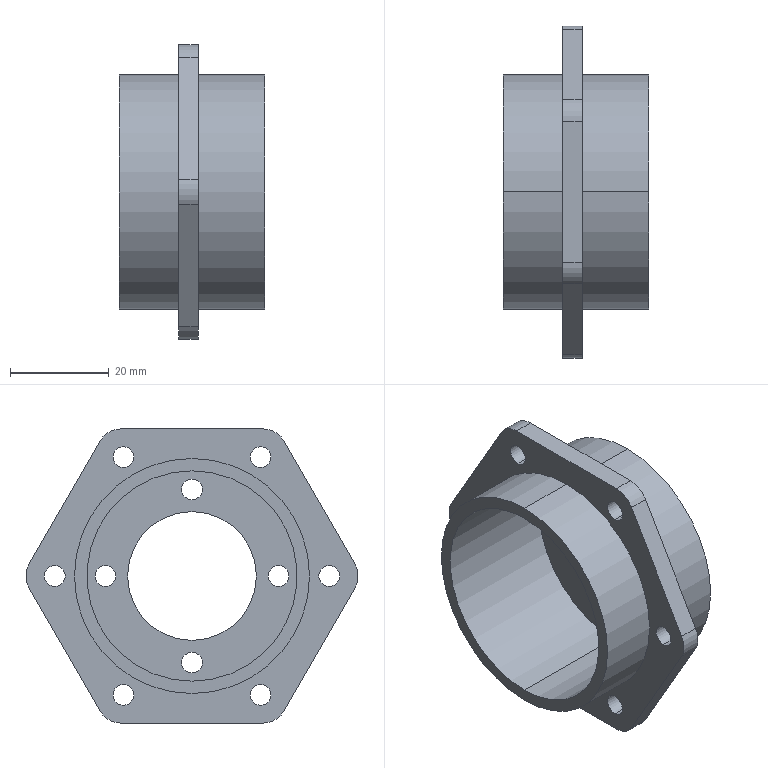Part | SolidWorks | features ICE 3, Fillet 1, Revolution 1 | 1 solid | 45 faces | box 29.45 x 67.158 x 59.5 mm | volume 18545 mm3 | cylinder 34 | plane 11 | commonest cylinder face diameters 4.2 x20 10 x6 47.5 x4 26.02 x2 42.5 x2
STEP:
#1=CARTESIAN_POINT('',(25.45,17.5,2.1));
#2=VERTEX_POINT('',#1);
#3=CARTESIAN_POINT('',(25.45,17.5,-2.1));
#4=VERTEX_POINT('',#3);
#5=CARTESIAN_POINT('',(25.45,17.5,0.));
#6=DIRECTION('',(1.,0.,0.));
#7=DIRECTION('',(0.,0.,-1.));
#8=AXIS2_PLACEMENT_3D('',#5,#6,#7);
#9=CIRCLE('',#8,2.1);
#10=EDGE_CURVE('',#2,#4,#9,.T.);
#11=ORIENTED_EDGE('',*,*,#10,.F.);
#12=CARTESIAN_POINT('',(29.45,17.5,2.1));
#13=VERTEX_POINT('',#12);
#14=CARTESIAN_POINT('',(0.,17.5,2.1));
#15=DIRECTION('',(1.,0.,0.));
#16=VECTOR('',#15,1000.);
#17=LINE('',#14,#16);
#18=EDGE_CURVE('',#2,#13,#17,.T.);
#19=ORIENTED_EDGE('',*,*,#18,.T.);
#20=CARTESIAN_POINT('',(29.45,17.5,-2.1));
#21=VERTEX_POINT('',#20);
#22=CARTESIAN_POINT('',(29.45,17.5,0.));
#23=DIRECTION('',(1.,0.,0.));
#24=DIRECTION('',(0.,0.,-1.));
#25=AXIS2_PLACEMENT_3D('',#22,#23,#24);
#26=CIRCLE('',#25,2.1);
#27=EDGE_CURVE('',#13,#21,#26,.T.);
#28=ORIENTED_EDGE('',*,*,#27,.T.);
#29=CARTESIAN_POINT('',(0.,17.5,-2.1));
#30=DIRECTION('',(1.,0.,0.));
#31=VECTOR('',#30,1000.);
#32=LINE('',#29,#31);
#33=EDGE_CURVE('',#4,#21,#32,.T.);
#34=ORIENTED_EDGE('',*,*,#33,.F.);
#35=EDGE_LOOP('',(#11,#19,#28,#34));
#36=FACE_OUTER_BOUND('',#35,.T.);
#37=CARTESIAN_POINT('',(0.,17.5,0.));
#38=DIRECTION('',(1.,0.,0.));
#39=DIRECTION('',(0.,0.,-1.));
#40=AXIS2_PLACEMENT_3D('',#37,#38,#39);
#41=CYLINDRICAL_SURFACE('',#40,2.1);
#42=ADVANCED_FACE('',(#36),#41,.F.);
#43=CARTESIAN_POINT('',(25.45,0.,-15.4));
#44=VERTEX_POINT('',#43);
#45=CARTESIAN_POINT('',(25.45,0.,-19.6));
#46=VERTEX_POINT('',#45);
#47=CARTESIAN_POINT('',(25.45,0.,-17.5));
#48=DIRECTION('',(1.,0.,0.));
#49=DIRECTION('',(0.,0.,-1.));
#50=AXIS2_PLACEMENT_3D('',#47,#48,#49);
#51=CIRCLE('',#50,2.1);
#52=EDGE_CURVE('',#44,#46,#51,.T.);
#53=ORIENTED_EDGE('',*,*,#52,.F.);
#54=CARTESIAN_POINT('',(29.45,0.,-15.4));
#55=VERTEX_POINT('',#54);
#56=CARTESIAN_POINT('',(0.,0.,-15.4));
#57=DIRECTION('',(1.,0.,0.));
#58=VECTOR('',#57,1000.);
#59=LINE('',#56,#58);
#60=EDGE_CURVE('',#44,#55,#59,.T.);
#61=ORIENTED_EDGE('',*,*,#60,.T.);
#62=CARTESIAN_POINT('',(29.45,0.,-19.6));
#63=VERTEX_POINT('',#62);
#64=CARTESIAN_POINT('',(29.45,0.,-17.5));
#65=DIRECTION('',(1.,0.,0.));
#66=DIRECTION('',(0.,0.,-1.));
#67=AXIS2_PLACEMENT_3D('',#64,#65,#66);
#68=CIRCLE('',#67,2.1);
#69=EDGE_CURVE('',#55,#63,#68,.T.);
#70=ORIENTED_EDGE('',*,*,#69,.T.);
#71=CARTESIAN_POINT('',(0.,0.,-19.6));
#72=DIRECTION('',(1.,0.,0.));
#73=VECTOR('',#72,1000.);
#74=LINE('',#71,#73);
#75=EDGE_CURVE('',#46,#63,#74,.T.);
#76=ORIENTED_EDGE('',*,*,#75,.F.);
#77=EDGE_LOOP('',(#53,#61,#70,#76));
#78=FACE_OUTER_BOUND('',#77,.T.);
#79=CARTESIAN_POINT('',(0.,0.,-17.5));
#80=DIRECTION('',(1.,0.,0.));
#81=DIRECTION('',(0.,0.,-1.));
#82=AXIS2_PLACEMENT_3D('',#79,#80,#81);
#83=CYLINDRICAL_SURFACE('',#82,2.1);
#84=ADVANCED_FACE('',(#78),#83,.F.);
#85=CARTESIAN_POINT('',(25.45,-17.5,2.1));
#86=VERTEX_POINT('',#85);
#87=CARTESIAN_POINT('',(25.45,-17.5,-2.1));
#88=VERTEX_POINT('',#87);
#89=CARTESIAN_POINT('',(25.45,-17.5,0.));
#90=DIRECTION('',(1.,0.,0.));
#91=DIRECTION('',(0.,0.,-1.));
#92=AXIS2_PLACEMENT_3D('',#89,#90,#91);
#93=CIRCLE('',#92,2.1);
#94=EDGE_CURVE('',#86,#88,#93,.T.);
#95=ORIENTED_EDGE('',*,*,#94,.F.);
#96=CARTESIAN_POINT('',(29.45,-17.5,2.1));
#97=VERTEX_POINT('',#96);
#98=CARTESIAN_POINT('',(0.,-17.5,2.1));
#99=DIRECTION('',(1.,0.,0.));
#100=VECTOR('',#99,1000.);
#101=LINE('',#98,#100);
#102=EDGE_CURVE('',#86,#97,#101,.T.);
#103=ORIENTED_EDGE('',*,*,#102,.T.);
#104=CARTESIAN_POINT('',(29.45,-17.5,-2.1));
#105=VERTEX_POINT('',#104);
#106=CARTESIAN_POINT('',(29.45,-17.5,0.));
#107=DIRECTION('',(1.,0.,0.));
#108=DIRECTION('',(0.,0.,-1.));
#109=AXIS2_PLACEMENT_3D('',#106,#107,#108);
#110=CIRCLE('',#109,2.1);
#111=EDGE_CURVE('',#97,#105,#110,.T.);
#112=ORIENTED_EDGE('',*,*,#111,.T.);
#113=CARTESIAN_POINT('',(0.,-17.5,-2.1));
#114=DIRECTION('',(1.,0.,0.));
#115=VECTOR('',#114,1000.);
#116=LINE('',#113,#115);
#117=EDGE_CURVE('',#88,#105,#116,.T.);
#118=ORIENTED_EDGE('',*,*,#117,.F.);
#119=EDGE_LOOP('',(#95,#103,#112,#118));
#120=FACE_OUTER_BOUND('',#119,.T.);
#121=CARTESIAN_POINT('',(0.,-17.5,0.));
#122=DIRECTION('',(1.,0.,0.));
#123=DIRECTION('',(0.,0.,-1.));
#124=AXIS2_PLACEMENT_3D('',#121,#122,#123);
#125=CYLINDRICAL_SURFACE('',#124,2.1);
#126=ADVANCED_FACE('',(#120),#125,.F.);
#127=CARTESIAN_POINT('',(25.45,0.,19.6));
#128=VERTEX_POINT('',#127);
#129=CARTESIAN_POINT('',(25.45,0.,15.4));
#130=VERTEX_POINT('',#129);
#131=CARTESIAN_POINT('',(25.45,0.,17.5));
#132=DIRECTION('',(1.,0.,0.));
#133=DIRECTION('',(0.,0.,-1.));
#134=AXIS2_PLACEMENT_3D('',#131,#132,#133);
#135=CIRCLE('',#134,2.1);
#136=EDGE_CURVE('',#128,#130,#135,.T.);
#137=ORIENTED_EDGE('',*,*,#136,.F.);
#138=CARTESIAN_POINT('',(29.45,0.,19.6));
#139=VERTEX_POINT('',#138);
#140=CARTESIAN_POINT('',(0.,0.,19.6));
#141=DIRECTION('',(1.,0.,0.));
#142=VECTOR('',#141,1000.);
#143=LINE('',#140,#142);
#144=EDGE_CURVE('',#128,#139,#143,.T.);
#145=ORIENTED_EDGE('',*,*,#144,.T.);
#146=CARTESIAN_POINT('',(29.45,0.,15.4));
#147=VERTEX_POINT('',#146);
#148=CARTESIAN_POINT('',(29.45,0.,17.5));
#149=DIRECTION('',(1.,0.,0.));
#150=DIRECTION('',(0.,0.,-1.));
#151=AXIS2_PLACEMENT_3D('',#148,#149,#150);
#152=CIRCLE('',#151,2.1);
#153=EDGE_CURVE('',#139,#147,#152,.T.);
#154=ORIENTED_EDGE('',*,*,#153,.T.);
#155=CARTESIAN_POINT('',(0.,0.,15.4));
#156=DIRECTION('',(1.,0.,0.));
#157=VECTOR('',#156,1000.);
#158=LINE('',#155,#157);
#159=EDGE_CURVE('',#130,#147,#158,.T.);
#160=ORIENTED_EDGE('',*,*,#159,.F.);
#161=EDGE_LOOP('',(#137,#145,#154,#160));
#162=FACE_OUTER_BOUND('',#161,.T.);
#163=CARTESIAN_POINT('',(0.,0.,17.5));
#164=DIRECTION('',(1.,0.,0.));
#165=DIRECTION('',(0.,0.,-1.));
#166=AXIS2_PLACEMENT_3D('',#163,#164,#165);
#167=CYLINDRICAL_SURFACE('',#166,2.1);
#168=ADVANCED_FACE('',(#162),#167,.F.);
#169=CARTESIAN_POINT('',(12.,13.875,-21.932));
#170=VERTEX_POINT('',#169);
#171=CARTESIAN_POINT('',(12.,13.875,-26.132));
#172=VERTEX_POINT('',#171);
#173=CARTESIAN_POINT('',(12.,13.875,-24.032));
#174=DIRECTION('',(1.,0.,0.));
#175=DIRECTION('',(0.,0.,-1.));
#176=AXIS2_PLACEMENT_3D('',#173,#174,#175);
#177=CIRCLE('',#176,2.1);
#178=EDGE_CURVE('',#170,#172,#177,.T.);
#179=ORIENTED_EDGE('',*,*,#178,.F.);
#180=CARTESIAN_POINT('',(16.,13.875,-21.932));
#181=VERTEX_POINT('',#180);
#182=CARTESIAN_POINT('',(0.,13.875,-21.932));
#183=DIRECTION('',(1.,0.,0.));
#184=VECTOR('',#183,1000.);
#185=LINE('',#182,#184);
#186=EDGE_CURVE('',#170,#181,#185,.T.);
#187=ORIENTED_EDGE('',*,*,#186,.T.);
#188=CARTESIAN_POINT('',(16.,13.875,-26.132));
#189=VERTEX_POINT('',#188);
#190=CARTESIAN_POINT('',(16.,13.875,-24.032));
#191=DIRECTION('',(1.,0.,0.));
#192=DIRECTION('',(0.,0.,-1.));
#193=AXIS2_PLACEMENT_3D('',#190,#191,#192);
#194=CIRCLE('',#193,2.1);
#195=EDGE_CURVE('',#181,#189,#194,.T.);
#196=ORIENTED_EDGE('',*,*,#195,.T.);
#197=CARTESIAN_POINT('',(0.,13.875,-26.132));
#198=DIRECTION('',(1.,0.,0.));
#199=VECTOR('',#198,1000.);
#200=LINE('',#197,#199);
#201=EDGE_CURVE('',#172,#189,#200,.T.);
#202=ORIENTED_EDGE('',*,*,#201,.F.);
#203=EDGE_LOOP('',(#179,#187,#196,#202));
#204=FACE_OUTER_BOUND('',#203,.T.);
#205=CARTESIAN_POINT('',(0.,13.875,-24.032));
#206=DIRECTION('',(1.,0.,0.));
#207=DIRECTION('',(0.,0.,-1.));
#208=AXIS2_PLACEMENT_3D('',#205,#206,#207);
#209=CYLINDRICAL_SURFACE('',#208,2.1);
#210=ADVANCED_FACE('',(#204),#209,.F.);
#211=CARTESIAN_POINT('',(12.,-13.875,-21.932));
#212=VERTEX_POINT('',#211);
#213=CARTESIAN_POINT('',(12.,-13.875,-26.132));
#214=VERTEX_POINT('',#213);
#215=CARTESIAN_POINT('',(12.,-13.875,-24.032));
#216=DIRECTION('',(1.,0.,0.));
#217=DIRECTION('',(0.,0.,-1.));
#218=AXIS2_PLACEMENT_3D('',#215,#216,#217);
#219=CIRCLE('',#218,2.1);
#220=EDGE_CURVE('',#212,#214,#219,.T.);
#221=ORIENTED_EDGE('',*,*,#220,.F.);
#222=CARTESIAN_POINT('',(16.,-13.875,-21.932));
#223=VERTEX_POINT('',#222);
#224=CARTESIAN_POINT('',(0.,-13.875,-21.932));
#225=DIRECTION('',(1.,0.,0.));
#226=VECTOR('',#225,1000.);
#227=LINE('',#224,#226);
#228=EDGE_CURVE('',#212,#223,#227,.T.);
#229=ORIENTED_EDGE('',*,*,#228,.T.);
#230=CARTESIAN_POINT('',(16.,-13.875,-26.132));
#231=VERTEX_POINT('',#230);
#232=CARTESIAN_POINT('',(16.,-13.875,-24.032));
#233=DIRECTION('',(1.,0.,0.));
#234=DIRECTION('',(0.,0.,-1.));
#235=AXIS2_PLACEMENT_3D('',#232,#233,#234);
#236=CIRCLE('',#235,2.1);
#237=EDGE_CURVE('',#223,#231,#236,.T.);
#238=ORIENTED_EDGE('',*,*,#237,.T.);
#239=CARTESIAN_POINT('',(0.,-13.875,-26.132));
#240=DIRECTION('',(1.,0.,0.));
#241=VECTOR('',#240,1000.);
#242=LINE('',#239,#241);
#243=EDGE_CURVE('',#214,#231,#242,.T.);
#244=ORIENTED_EDGE('',*,*,#243,.F.);
#245=EDGE_LOOP('',(#221,#229,#238,#244));
#246=FACE_OUTER_BOUND('',#245,.T.);
#247=CARTESIAN_POINT('',(0.,-13.875,-24.032));
#248=DIRECTION('',(1.,0.,0.));
#249=DIRECTION('',(0.,0.,-1.));
#250=AXIS2_PLACEMENT_3D('',#247,#248,#249);
#251=CYLINDRICAL_SURFACE('',#250,2.1);
#252=ADVANCED_FACE('',(#246),#251,.F.);
#253=CARTESIAN_POINT('',(12.,-27.75,2.1));
#254=VERTEX_POINT('',#253);
#255=CARTESIAN_POINT('',(12.,-27.75,-2.1));
#256=VERTEX_POINT('',#255);
#257=CARTESIAN_POINT('',(12.,-27.75,0.));
#258=DIRECTION('',(1.,0.,0.));
#259=DIRECTION('',(0.,0.,-1.));
#260=AXIS2_PLACEMENT_3D('',#257,#258,#259);
#261=CIRCLE('',#260,2.1);
#262=EDGE_CURVE('',#254,#256,#261,.T.);
#263=ORIENTED_EDGE('',*,*,#262,.F.);
#264=CARTESIAN_POINT('',(16.,-27.75,2.1));
#265=VERTEX_POINT('',#264);
#266=CARTESIAN_POINT('',(0.,-27.75,2.1));
#267=DIRECTION('',(1.,0.,0.));
#268=VECTOR('',#267,1000.);
#269=LINE('',#266,#268);
#270=EDGE_CURVE('',#254,#265,#269,.T.);
#271=ORIENTED_EDGE('',*,*,#270,.T.);
#272=CARTESIAN_POINT('',(16.,-27.75,-2.1));
#273=VERTEX_POINT('',#272);
#274=CARTESIAN_POINT('',(16.,-27.75,0.));
#275=DIRECTION('',(1.,0.,0.));
#276=DIRECTION('',(0.,0.,-1.));
#277=AXIS2_PLACEMENT_3D('',#274,#275,#276);
#278=CIRCLE('',#277,2.1);
#279=EDGE_CURVE('',#265,#273,#278,.T.);
#280=ORIENTED_EDGE('',*,*,#279,.T.);
#281=CARTESIAN_POINT('',(0.,-27.75,-2.1));
#282=DIRECTION('',(1.,0.,0.));
#283=VECTOR('',#282,1000.);
#284=LINE('',#281,#283);
#285=EDGE_CURVE('',#256,#273,#284,.T.);
#286=ORIENTED_EDGE('',*,*,#285,.F.);
#287=EDGE_LOOP('',(#263,#271,#280,#286));
#288=FACE_OUTER_BOUND('',#287,.T.);
#289=CARTESIAN_POINT('',(0.,-27.75,0.));
#290=DIRECTION('',(1.,0.,0.));
#291=DIRECTION('',(0.,0.,-1.));
#292=AXIS2_PLACEMENT_3D('',#289,#290,#291);
#293=CYLINDRICAL_SURFACE('',#292,2.1);
#294=ADVANCED_FACE('',(#288),#293,.F.);
#295=CARTESIAN_POINT('',(12.,-13.875,26.132));
#296=VERTEX_POINT('',#295);
#297=CARTESIAN_POINT('',(12.,-13.875,21.932));
#298=VERTEX_POINT('',#297);
#299=CARTESIAN_POINT('',(12.,-13.875,24.032));
#300=DIRECTION('',(1.,0.,0.));
#301=DIRECTION('',(0.,0.,-1.));
#302=AXIS2_PLACEMENT_3D('',#299,#300,#301);
#303=CIRCLE('',#302,2.1);
#304=EDGE_CURVE('',#296,#298,#303,.T.);
#305=ORIENTED_EDGE('',*,*,#304,.F.);
#306=CARTESIAN_POINT('',(16.,-13.875,26.132));
#307=VERTEX_POINT('',#306);
#308=CARTESIAN_POINT('',(0.,-13.875,26.132));
#309=DIRECTION('',(1.,0.,0.));
#310=VECTOR('',#309,1000.);
#311=LINE('',#308,#310);
#312=EDGE_CURVE('',#296,#307,#311,.T.);
#313=ORIENTED_EDGE('',*,*,#312,.T.);
#314=CARTESIAN_POINT('',(16.,-13.875,21.932));
#315=VERTEX_POINT('',#314);
#316=CARTESIAN_POINT('',(16.,-13.875,24.032));
#317=DIRECTION('',(1.,0.,0.));
#318=DIRECTION('',(0.,0.,-1.));
#319=AXIS2_PLACEMENT_3D('',#316,#317,#318);
#320=CIRCLE('',#319,2.1);
#321=EDGE_CURVE('',#307,#315,#320,.T.);
#322=ORIENTED_EDGE('',*,*,#321,.T.);
#323=CARTESIAN_POINT('',(0.,-13.875,21.932));
#324=DIRECTION('',(1.,0.,0.));
#325=VECTOR('',#324,1000.);
#326=LINE('',#323,#325);
#327=EDGE_CURVE('',#298,#315,#326,.T.);
#328=ORIENTED_EDGE('',*,*,#327,.F.);
#329=EDGE_LOOP('',(#305,#313,#322,#328));
#330=FACE_OUTER_BOUND('',#329,.T.);
#331=CARTESIAN_POINT('',(0.,-13.875,24.032));
#332=DIRECTION('',(1.,0.,0.));
#333=DIRECTION('',(0.,0.,-1.));
#334=AXIS2_PLACEMENT_3D('',#331,#332,#333);
#335=CYLINDRICAL_SURFACE('',#334,2.1);
#336=ADVANCED_FACE('',(#330),#335,.F.);
#337=CARTESIAN_POINT('',(12.,13.875,26.132));
#338=VERTEX_POINT('',#337);
#339=CARTESIAN_POINT('',(12.,13.875,21.932));
#340=VERTEX_POINT('',#339);
#341=CARTESIAN_POINT('',(12.,13.875,24.032));
#342=DIRECTION('',(1.,0.,0.));
#343=DIRECTION('',(0.,0.,-1.));
#344=AXIS2_PLACEMENT_3D('',#341,#342,#343);
#345=CIRCLE('',#344,2.1);
#346=EDGE_CURVE('',#338,#340,#345,.T.);
#347=ORIENTED_EDGE('',*,*,#346,.F.);
#348=CARTESIAN_POINT('',(16.,13.875,26.132));
#349=VERTEX_POINT('',#348);
#350=CARTESIAN_POINT('',(0.,13.875,26.132));
#351=DIRECTION('',(1.,0.,0.));
#352=VECTOR('',#351,1000.);
#353=LINE('',#350,#352);
#354=EDGE_CURVE('',#338,#349,#353,.T.);
#355=ORIENTED_EDGE('',*,*,#354,.T.);
#356=CARTESIAN_POINT('',(16.,13.875,21.932));
#357=VERTEX_POINT('',#356);
#358=CARTESIAN_POINT('',(16.,13.875,24.032));
#359=DIRECTION('',(1.,0.,0.));
#360=DIRECTION('',(0.,0.,-1.));
#361=AXIS2_PLACEMENT_3D('',#358,#359,#360);
#362=CIRCLE('',#361,2.1);
#363=EDGE_CURVE('',#349,#357,#362,.T.);
#364=ORIENTED_EDGE('',*,*,#363,.T.);
#365=CARTESIAN_POINT('',(0.,13.875,21.932));
#366=DIRECTION('',(1.,0.,0.));
#367=VECTOR('',#366,1000.);
#368=LINE('',#365,#367);
#369=EDGE_CURVE('',#340,#357,#368,.T.);
#370=ORIENTED_EDGE('',*,*,#369,.F.);
#371=EDGE_LOOP('',(#347,#355,#364,#370));
#372=FACE_OUTER_BOUND('',#371,.T.);
#373=CARTESIAN_POINT('',(0.,13.875,24.032));
#374=DIRECTION('',(1.,0.,0.));
#375=DIRECTION('',(0.,0.,-1.));
#376=AXIS2_PLACEMENT_3D('',#373,#374,#375);
#377=CYLINDRICAL_SURFACE('',#376,2.1);
#378=ADVANCED_FACE('',(#372),#377,.F.);
#379=CARTESIAN_POINT('',(12.,27.75,2.1));
#380=VERTEX_POINT('',#379);
#381=CARTESIAN_POINT('',(12.,27.75,-2.1));
#382=VERTEX_POINT('',#381);
#383=CARTESIAN_POINT('',(12.,27.75,0.));
#384=DIRECTION('',(1.,0.,0.));
#385=DIRECTION('',(0.,0.,-1.));
#386=AXIS2_PLACEMENT_3D('',#383,#384,#385);
#387=CIRCLE('',#386,2.1);
#388=EDGE_CURVE('',#380,#382,#387,.T.);
#389=ORIENTED_EDGE('',*,*,#388,.F.);
#390=CARTESIAN_POINT('',(16.,27.75,2.1));
#391=VERTEX_POINT('',#390);
#392=CARTESIAN_POINT('',(0.,27.75,2.1));
#393=DIRECTION('',(1.,0.,0.));
#394=VECTOR('',#393,1000.);
#395=LINE('',#392,#394);
#396=EDGE_CURVE('',#380,#391,#395,.T.);
#397=ORIENTED_EDGE('',*,*,#396,.T.);
#398=CARTESIAN_POINT('',(16.,27.75,-2.1));
#399=VERTEX_POINT('',#398);
#400=CARTESIAN_POINT('',(16.,27.75,0.));
#401=DIRECTION('',(1.,0.,0.));
#402=DIRECTION('',(0.,0.,-1.));
#403=AXIS2_PLACEMENT_3D('',#400,#401,#402);
#404=CIRCLE('',#403,2.1);
#405=EDGE_CURVE('',#391,#399,#404,.T.);
#406=ORIENTED_EDGE('',*,*,#405,.T.);
#407=CARTESIAN_POINT('',(0.,27.75,-2.1));
#408=DIRECTION('',(1.,0.,0.));
#409=VECTOR('',#408,1000.);
#410=LINE('',#407,#409);
#411=EDGE_CURVE('',#382,#399,#410,.T.);
#412=ORIENTED_EDGE('',*,*,#411,.F.);
#413=EDGE_LOOP('',(#389,#397,#406,#412));
#414=FACE_OUTER_BOUND('',#413,.T.);
#415=CARTESIAN_POINT('',(0.,27.75,0.));
#416=DIRECTION('',(1.,0.,0.));
#417=DIRECTION('',(0.,0.,-1.));
#418=AXIS2_PLACEMENT_3D('',#415,#416,#417);
#419=CYLINDRICAL_SURFACE('',#418,2.1);
#420=ADVANCED_FACE('',(#414),#419,.F.);
#421=CARTESIAN_POINT('',(29.45,0.,-13.01));
#422=VERTEX_POINT('',#421);
#423=CARTESIAN_POINT('',(29.45,0.,13.01));
#424=VERTEX_POINT('',#423);
#425=CARTESIAN_POINT('',(29.45,0.,0.));
#426=DIRECTION('',(-1.,0.,0.));
#427=DIRECTION('',(0.,0.,1.));
#428=AXIS2_PLACEMENT_3D('',#425,#426,#427);
#429=CIRCLE('',#428,13.01);
#430=EDGE_CURVE('',#422,#424,#429,.T.);
#431=ORIENTED_EDGE('',*,*,#430,.F.);
#432=CARTESIAN_POINT('',(25.45,0.,-13.01));
#433=VERTEX_POINT('',#432);
#434=CARTESIAN_POINT('',(-873.27,0.,-13.01));
#435=DIRECTION('',(-1.,0.,0.));
#436=VECTOR('',#435,1000.);
#437=LINE('',#434,#436);
#438=EDGE_CURVE('',#422,#433,#437,.T.);
#439=ORIENTED_EDGE('',*,*,#438,.T.);
#440=CARTESIAN_POINT('',(25.45,0.,13.01));
#441=VERTEX_POINT('',#440);
#442=CARTESIAN_POINT('',(25.45,0.,0.));
#443=DIRECTION('',(-1.,0.,0.));
#444=DIRECTION('',(0.,0.,1.));
#445=AXIS2_PLACEMENT_3D('',#442,#443,#444);
#446=CIRCLE('',#445,13.01);
#447=EDGE_CURVE('',#433,#441,#446,.T.);
#448=ORIENTED_EDGE('',*,*,#447,.T.);
#449=CARTESIAN_POINT('',(-873.27,0.,13.01));
#450=DIRECTION('',(-1.,0.,0.));
#451=VECTOR('',#450,1000.);
#452=LINE('',#449,#451);
#453=EDGE_CURVE('',#424,#441,#452,.T.);
#454=ORIENTED_EDGE('',*,*,#453,.F.);
#455=EDGE_LOOP('',(#431,#439,#448,#454));
#456=FACE_OUTER_BOUND('',#455,.T.);
#457=CARTESIAN_POINT('',(-873.27,0.,0.));
#458=DIRECTION('',(-1.,0.,0.));
#459=DIRECTION('',(0.,0.,1.));
#460=AXIS2_PLACEMENT_3D('',#457,#458,#459);
#461=CYLINDRICAL_SURFACE('',#460,13.01);
#462=ADVANCED_FACE('',(#456),#461,.F.);
#463=CARTESIAN_POINT('',(29.45,0.,23.75));
#464=VERTEX_POINT('',#463);
#465=CARTESIAN_POINT('',(29.45,0.,-23.75));
#466=VERTEX_POINT('',#465);
#467=CARTESIAN_POINT('',(29.45,0.,0.));
#468=DIRECTION('',(-1.,0.,0.));
#469=DIRECTION('',(0.,0.,1.));
#470=AXIS2_PLACEMENT_3D('',#467,#468,#469);
#471=CIRCLE('',#470,23.75);
#472=EDGE_CURVE('',#464,#466,#471,.T.);
#473=ORIENTED_EDGE('',*,*,#472,.T.);
#474=CARTESIAN_POINT('',(16.,0.,-23.75));
#475=VERTEX_POINT('',#474);
#476=CARTESIAN_POINT('',(-873.27,0.,-23.75));
#477=DIRECTION('',(-1.,0.,0.));
#478=VECTOR('',#477,1000.);
#479=LINE('',#476,#478);
#480=EDGE_CURVE('',#466,#475,#479,.T.);
#481=ORIENTED_EDGE('',*,*,#480,.T.);
#482=CARTESIAN_POINT('',(16.,0.,23.75));
#483=VERTEX_POINT('',#482);
#484=CARTESIAN_POINT('',(16.,0.,0.));
#485=DIRECTION('',(-1.,0.,0.));
#486=DIRECTION('',(0.,0.,1.));
#487=AXIS2_PLACEMENT_3D('',#484,#485,#486);
#488=CIRCLE('',#487,23.75);
#489=EDGE_CURVE('',#483,#475,#488,.T.);
#490=ORIENTED_EDGE('',*,*,#489,.F.);
#491=CARTESIAN_POINT('',(-873.27,0.,23.75));
#492=DIRECTION('',(-1.,0.,0.));
#493=VECTOR('',#492,1000.);
#494=LINE('',#491,#493);
#495=EDGE_CURVE('',#464,#483,#494,.T.);
#496=ORIENTED_EDGE('',*,*,#495,.F.);
#497=EDGE_LOOP('',(#473,#481,#490,#496));
#498=FACE_OUTER_BOUND('',#497,.T.);
#499=CARTESIAN_POINT('',(-873.27,0.,0.));
#500=DIRECTION('',(-1.,0.,0.));
#501=DIRECTION('',(0.,0.,1.));
#502=AXIS2_PLACEMENT_3D('',#499,#500,#501);
#503=CYLINDRICAL_SURFACE('',#502,23.75);
#504=ADVANCED_FACE('',(#498),#503,.T.);
#505=CARTESIAN_POINT('',(12.,0.,23.75));
#506=VERTEX_POINT('',#505);
#507=CARTESIAN_POINT('',(12.,0.,-23.75));
#508=VERTEX_POINT('',#507);
#509=CARTESIAN_POINT('',(12.,0.,0.));
#510=DIRECTION('',(-1.,0.,0.));
#511=DIRECTION('',(0.,0.,1.));
#512=AXIS2_PLACEMENT_3D('',#509,#510,#511);
#513=CIRCLE('',#512,23.75);
#514=EDGE_CURVE('',#506,#508,#513,.T.);
#515=ORIENTED_EDGE('',*,*,#514,.T.);
#516=CARTESIAN_POINT('',(0.,0.,-23.75));
#517=VERTEX_POINT('',#516);
#518=CARTESIAN_POINT('',(-873.27,0.,-23.75));
#519=DIRECTION('',(-1.,0.,0.));
#520=VECTOR('',#519,1000.);
#521=LINE('',#518,#520);
#522=EDGE_CURVE('',#508,#517,#521,.T.);
#523=ORIENTED_EDGE('',*,*,#522,.T.);
#524=CARTESIAN_POINT('',(0.,0.,23.75));
#525=VERTEX_POINT('',#524);
#526=CARTESIAN_POINT('',(0.,0.,0.));
#527=DIRECTION('',(-1.,0.,0.));
#528=DIRECTION('',(0.,0.,1.));
#529=AXIS2_PLACEMENT_3D('',#526,#527,#528);
#530=CIRCLE('',#529,23.75);
#531=EDGE_CURVE('',#525,#517,#530,.T.);
#532=ORIENTED_EDGE('',*,*,#531,.F.);
#533=CARTESIAN_POINT('',(-873.27,0.,23.75));
#534=DIRECTION('',(-1.,0.,0.));
#535=VECTOR('',#534,1000.);
#536=LINE('',#533,#535);
#537=EDGE_CURVE('',#506,#525,#536,.T.);
#538=ORIENTED_EDGE('',*,*,#537,.F.);
#539=EDGE_LOOP('',(#515,#523,#532,#538));
#540=FACE_OUTER_BOUND('',#539,.T.);
#541=CARTESIAN_POINT('',(-873.27,0.,0.));
#542=DIRECTION('',(-1.,0.,0.));
#543=DIRECTION('',(0.,0.,1.));
#544=AXIS2_PLACEMENT_3D('',#541,#542,#543);
#545=CYLINDRICAL_SURFACE('',#544,23.75);
#546=ADVANCED_FACE('',(#540),#545,.T.);
#547=CARTESIAN_POINT('',(25.45,0.,-21.25));
#548=VERTEX_POINT('',#547);
#549=CARTESIAN_POINT('',(25.45,0.,21.25));
#550=VERTEX_POINT('',#549);
#551=CARTESIAN_POINT('',(25.45,0.,0.));
#552=DIRECTION('',(-1.,0.,0.));
#553=DIRECTION('',(0.,0.,1.));
#554=AXIS2_PLACEMENT_3D('',#551,#552,#553);
#555=CIRCLE('',#554,21.25);
#556=EDGE_CURVE('',#548,#550,#555,.T.);
#557=ORIENTED_EDGE('',*,*,#556,.F.);
#558=CARTESIAN_POINT('',(0.,0.,-21.25));
#559=VERTEX_POINT('',#558);
#560=CARTESIAN_POINT('',(-873.27,0.,-21.25));
#561=DIRECTION('',(-1.,0.,0.));
#562=VECTOR('',#561,1000.);
#563=LINE('',#560,#562);
#564=EDGE_CURVE('',#548,#559,#563,.T.);
#565=ORIENTED_EDGE('',*,*,#564,.T.);
#566=CARTESIAN_POINT('',(0.,0.,21.25));
#567=VERTEX_POINT('',#566);
#568=CARTESIAN_POINT('',(0.,0.,0.));
#569=DIRECTION('',(-1.,0.,0.));
#570=DIRECTION('',(0.,0.,1.));
#571=AXIS2_PLACEMENT_3D('',#568,#569,#570);
#572=CIRCLE('',#571,21.25);
#573=EDGE_CURVE('',#559,#567,#572,.T.);
#574=ORIENTED_EDGE('',*,*,#573,.T.);
#575=CARTESIAN_POINT('',(-873.27,0.,21.25));
#576=DIRECTION('',(-1.,0.,0.));
#577=VECTOR('',#576,1000.);
#578=LINE('',#575,#577);
#579=EDGE_CURVE('',#550,#567,#578,.T.);
#580=ORIENTED_EDGE('',*,*,#579,.F.);
#581=EDGE_LOOP('',(#557,#565,#574,#580));
#582=FACE_OUTER_BOUND('',#581,.T.);
#583=CARTESIAN_POINT('',(-873.27,0.,0.));
#584=DIRECTION('',(-1.,0.,0.));
#585=DIRECTION('',(0.,0.,1.));
#586=AXIS2_PLACEMENT_3D('',#583,#584,#585);
#587=CYLINDRICAL_SURFACE('',#586,21.25);
#588=ADVANCED_FACE('',(#582),#587,.F.);
#589=CARTESIAN_POINT('',(12.,27.75,0.));
#590=DIRECTION('',(1.,0.,0.));
#591=DIRECTION('',(0.,0.,-1.));
#592=AXIS2_PLACEMENT_3D('',#589,#590,#591);
#593=CIRCLE('',#592,2.1);
#594=EDGE_CURVE('',#382,#380,#593,.T.);
#595=ORIENTED_EDGE('',*,*,#594,.T.);
#596=ORIENTED_EDGE('',*,*,#388,.T.);
#597=EDGE_LOOP('',(#595,#596));
#598=FACE_BOUND('',#597,.T.);
#599=ORIENTED_EDGE('',*,*,#514,.F.);
#600=CARTESIAN_POINT('',(12.,0.,0.));
#601=DIRECTION('',(-1.,0.,0.));
#602=DIRECTION('',(0.,0.,1.));
#603=AXIS2_PLACEMENT_3D('',#600,#601,#602);
#604=CIRCLE('',#603,23.75);
#605=EDGE_CURVE('',#508,#506,#604,.T.);
#606=ORIENTED_EDGE('',*,*,#605,.F.);
#607=EDGE_LOOP('',(#599,#606));
#608=FACE_BOUND('',#607,.T.);
#609=CARTESIAN_POINT('',(12.,13.875,24.032));
#610=DIRECTION('',(1.,0.,0.));
#611=DIRECTION('',(0.,0.,-1.));
#612=AXIS2_PLACEMENT_3D('',#609,#610,#611);
#613=CIRCLE('',#612,2.1);
#614=EDGE_CURVE('',#340,#338,#613,.T.);
#615=ORIENTED_EDGE('',*,*,#614,.T.);
#616=ORIENTED_EDGE('',*,*,#346,.T.);
#617=EDGE_LOOP('',(#615,#616));
#618=FACE_BOUND('',#617,.T.);
#619=CARTESIAN_POINT('',(12.,-13.875,24.032));
#620=DIRECTION('',(1.,0.,0.));
#621=DIRECTION('',(0.,0.,-1.));
#622=AXIS2_PLACEMENT_3D('',#619,#620,#621);
#623=CIRCLE('',#622,2.1);
#624=EDGE_CURVE('',#298,#296,#623,.T.);
#625=ORIENTED_EDGE('',*,*,#624,.T.);
#626=ORIENTED_EDGE('',*,*,#304,.T.);
#627=EDGE_LOOP('',(#625,#626));
#628=FACE_BOUND('',#627,.T.);
#629=CARTESIAN_POINT('',(12.,-27.75,0.));
#630=DIRECTION('',(1.,0.,0.));
#631=DIRECTION('',(0.,0.,-1.));
#632=AXIS2_PLACEMENT_3D('',#629,#630,#631);
#633=CIRCLE('',#632,2.1);
#634=EDGE_CURVE('',#256,#254,#633,.T.);
#635=ORIENTED_EDGE('',*,*,#634,.T.);
#636=ORIENTED_EDGE('',*,*,#262,.T.);
#637=EDGE_LOOP('',(#635,#636));
#638=FACE_BOUND('',#637,.T.);
#639=CARTESIAN_POINT('',(12.,-13.875,-24.032));
#640=DIRECTION('',(1.,0.,0.));
#641=DIRECTION('',(0.,0.,-1.));
#642=AXIS2_PLACEMENT_3D('',#639,#640,#641);
#643=CIRCLE('',#642,2.1);
#644=EDGE_CURVE('',#214,#212,#643,.T.);
#645=ORIENTED_EDGE('',*,*,#644,.T.);
#646=ORIENTED_EDGE('',*,*,#220,.T.);
#647=EDGE_LOOP('',(#645,#646));
#648=FACE_BOUND('',#647,.T.);
#649=CARTESIAN_POINT('',(12.,13.875,-24.032));
#650=DIRECTION('',(1.,0.,0.));
#651=DIRECTION('',(0.,0.,-1.));
#652=AXIS2_PLACEMENT_3D('',#649,#650,#651);
#653=CIRCLE('',#652,2.1);
#654=EDGE_CURVE('',#172,#170,#653,.T.);
#655=ORIENTED_EDGE('',*,*,#654,.T.);
#656=ORIENTED_EDGE('',*,*,#178,.T.);
#657=EDGE_LOOP('',(#655,#656));
#658=FACE_BOUND('',#657,.T.);
#659=CARTESIAN_POINT('',(12.,-18.62,27.25));
#660=VERTEX_POINT('',#659);
#661=CARTESIAN_POINT('',(12.,-32.909,2.5));
#662=VERTEX_POINT('',#661);
#663=CARTESIAN_POINT('',(12.,-36.048,-2.937));
#664=DIRECTION('',(0.,-0.5,-0.866));
#665=VECTOR('',#664,1000.);
#666=LINE('',#663,#665);
#667=EDGE_CURVE('',#660,#662,#666,.T.);
#668=ORIENTED_EDGE('',*,*,#667,.F.);
#669=CARTESIAN_POINT('',(12.,-14.289,29.75));
#670=VERTEX_POINT('',#669);
#671=CARTESIAN_POINT('',(12.,-14.289,24.75));
#672=DIRECTION('',(-1.,0.,0.));
#673=DIRECTION('',(0.,0.,-1.));
#674=AXIS2_PLACEMENT_3D('',#671,#672,#673);
#675=CIRCLE('',#674,5.);
#676=EDGE_CURVE('',#660,#670,#675,.T.);
#677=ORIENTED_EDGE('',*,*,#676,.T.);
#678=CARTESIAN_POINT('',(12.,14.289,29.75));
#679=VERTEX_POINT('',#678);
#680=CARTESIAN_POINT('',(12.,0.,29.75));
#681=DIRECTION('',(0.,-1.,0.));
#682=VECTOR('',#681,1000.);
#683=LINE('',#680,#682);
#684=EDGE_CURVE('',#679,#670,#683,.T.);
#685=ORIENTED_EDGE('',*,*,#684,.F.);
#686=CARTESIAN_POINT('',(12.,18.62,27.25));
#687=VERTEX_POINT('',#686);
#688=CARTESIAN_POINT('',(12.,14.289,24.75));
#689=DIRECTION('',(-1.,0.,0.));
#690=DIRECTION('',(0.,0.,-1.));
#691=AXIS2_PLACEMENT_3D('',#688,#689,#690);
#692=CIRCLE('',#691,5.);
#693=EDGE_CURVE('',#679,#687,#692,.T.);
#694=ORIENTED_EDGE('',*,*,#693,.T.);
#695=CARTESIAN_POINT('',(12.,32.909,2.5));
#696=VERTEX_POINT('',#695);
#697=CARTESIAN_POINT('',(12.,36.048,-2.938));
#698=DIRECTION('',(0.,-0.5,0.866));
#699=VECTOR('',#698,1000.);
#700=LINE('',#697,#699);
#701=EDGE_CURVE('',#696,#687,#700,.T.);
#702=ORIENTED_EDGE('',*,*,#701,.F.);
#703=CARTESIAN_POINT('',(12.,32.909,-2.5));
#704=VERTEX_POINT('',#703);
#705=CARTESIAN_POINT('',(12.,28.579,0.));
#706=DIRECTION('',(-1.,0.,0.));
#707=DIRECTION('',(0.,0.,-1.));
#708=AXIS2_PLACEMENT_3D('',#705,#706,#707);
#709=CIRCLE('',#708,5.);
#710=EDGE_CURVE('',#696,#704,#709,.T.);
#711=ORIENTED_EDGE('',*,*,#710,.T.);
#712=CARTESIAN_POINT('',(12.,18.62,-27.25));
#713=VERTEX_POINT('',#712);
#714=CARTESIAN_POINT('',(12.,15.48,-32.688));
#715=DIRECTION('',(0.,0.5,0.866));
#716=VECTOR('',#715,1000.);
#717=LINE('',#714,#716);
#718=EDGE_CURVE('',#713,#704,#717,.T.);
#719=ORIENTED_EDGE('',*,*,#718,.F.);
#720=CARTESIAN_POINT('',(12.,14.289,-29.75));
#721=VERTEX_POINT('',#720);
#722=CARTESIAN_POINT('',(12.,14.289,-24.75));
#723=DIRECTION('',(-1.,0.,0.));
#724=DIRECTION('',(0.,0.,-1.));
#725=AXIS2_PLACEMENT_3D('',#722,#723,#724);
#726=CIRCLE('',#725,5.);
#727=EDGE_CURVE('',#713,#721,#726,.T.);
#728=ORIENTED_EDGE('',*,*,#727,.T.);
#729=CARTESIAN_POINT('',(12.,-14.289,-29.75));
#730=VERTEX_POINT('',#729);
#731=CARTESIAN_POINT('',(12.,0.,-29.75));
#732=DIRECTION('',(0.,1.,0.));
#733=VECTOR('',#732,1000.);
#734=LINE('',#731,#733);
#735=EDGE_CURVE('',#730,#721,#734,.T.);
#736=ORIENTED_EDGE('',*,*,#735,.F.);
#737=CARTESIAN_POINT('',(12.,-18.62,-27.25));
#738=VERTEX_POINT('',#737);
#739=CARTESIAN_POINT('',(12.,-14.289,-24.75));
#740=DIRECTION('',(-1.,0.,0.));
#741=DIRECTION('',(0.,0.,-1.));
#742=AXIS2_PLACEMENT_3D('',#739,#740,#741);
#743=CIRCLE('',#742,5.);
#744=EDGE_CURVE('',#730,#738,#743,.T.);
#745=ORIENTED_EDGE('',*,*,#744,.T.);
#746=CARTESIAN_POINT('',(12.,-32.909,-2.5));
#747=VERTEX_POINT('',#746);
#748=CARTESIAN_POINT('',(12.,-15.48,-32.688));
#749=DIRECTION('',(0.,0.5,-0.866));
#750=VECTOR('',#749,1000.);
#751=LINE('',#748,#750);
#752=EDGE_CURVE('',#747,#738,#751,.T.);
#753=ORIENTED_EDGE('',*,*,#752,.F.);
#754=CARTESIAN_POINT('',(12.,-28.579,0.));
#755=DIRECTION('',(-1.,0.,0.));
#756=DIRECTION('',(0.,0.,-1.));
#757=AXIS2_PLACEMENT_3D('',#754,#755,#756);
#758=CIRCLE('',#757,5.);
#759=EDGE_CURVE('',#747,#662,#758,.T.);
#760=ORIENTED_EDGE('',*,*,#759,.T.);
#761=EDGE_LOOP('',(#668,#677,#685,#694,#702,#711,#719,#728,#736,#745,#753,#760));
#762=FACE_OUTER_BOUND('',#761,.T.);
#763=CARTESIAN_POINT('',(12.,0.,-23.75));
#764=DIRECTION('',(1.,0.,0.));
#765=DIRECTION('',(0.,0.,-1.));
#766=AXIS2_PLACEMENT_3D('',#763,#764,#765);
#767=PLANE('',#766);
#768=ADVANCED_FACE('',(#598,#608,#618,#628,#638,#648,#658,#762),#767,.F.);
#769=CARTESIAN_POINT('',(16.,27.75,0.));
#770=DIRECTION('',(1.,0.,0.));
#771=DIRECTION('',(0.,0.,-1.));
#772=AXIS2_PLACEMENT_3D('',#769,#770,#771);
#773=CIRCLE('',#772,2.1);
#774=EDGE_CURVE('',#399,#391,#773,.T.);
#775=ORIENTED_EDGE('',*,*,#774,.F.);
#776=ORIENTED_EDGE('',*,*,#405,.F.);
#777=EDGE_LOOP('',(#775,#776));
#778=FACE_BOUND('',#777,.T.);
#779=ORIENTED_EDGE('',*,*,#489,.T.);
#780=CARTESIAN_POINT('',(16.,0.,0.));
#781=DIRECTION('',(-1.,0.,0.));
#782=DIRECTION('',(0.,0.,1.));
#783=AXIS2_PLACEMENT_3D('',#780,#781,#782);
#784=CIRCLE('',#783,23.75);
#785=EDGE_CURVE('',#475,#483,#784,.T.);
#786=ORIENTED_EDGE('',*,*,#785,.T.);
#787=EDGE_LOOP('',(#779,#786));
#788=FACE_BOUND('',#787,.T.);
#789=CARTESIAN_POINT('',(16.,13.875,24.032));
#790=DIRECTION('',(1.,0.,0.));
#791=DIRECTION('',(0.,0.,-1.));
#792=AXIS2_PLACEMENT_3D('',#789,#790,#791);
#793=CIRCLE('',#792,2.1);
#794=EDGE_CURVE('',#357,#349,#793,.T.);
#795=ORIENTED_EDGE('',*,*,#794,.F.);
#796=ORIENTED_EDGE('',*,*,#363,.F.);
#797=EDGE_LOOP('',(#795,#796));
#798=FACE_BOUND('',#797,.T.);
#799=CARTESIAN_POINT('',(16.,-13.875,24.032));
#800=DIRECTION('',(1.,0.,0.));
#801=DIRECTION('',(0.,0.,-1.));
#802=AXIS2_PLACEMENT_3D('',#799,#800,#801);
#803=CIRCLE('',#802,2.1);
#804=EDGE_CURVE('',#315,#307,#803,.T.);
#805=ORIENTED_EDGE('',*,*,#804,.F.);
#806=ORIENTED_EDGE('',*,*,#321,.F.);
#807=EDGE_LOOP('',(#805,#806));
#808=FACE_BOUND('',#807,.T.);
#809=CARTESIAN_POINT('',(16.,-27.75,0.));
#810=DIRECTION('',(1.,0.,0.));
#811=DIRECTION('',(0.,0.,-1.));
#812=AXIS2_PLACEMENT_3D('',#809,#810,#811);
#813=CIRCLE('',#812,2.1);
#814=EDGE_CURVE('',#273,#265,#813,.T.);
#815=ORIENTED_EDGE('',*,*,#814,.F.);
#816=ORIENTED_EDGE('',*,*,#279,.F.);
#817=EDGE_LOOP('',(#815,#816));
#818=FACE_BOUND('',#817,.T.);
#819=CARTESIAN_POINT('',(16.,-13.875,-24.032));
#820=DIRECTION('',(1.,0.,0.));
#821=DIRECTION('',(0.,0.,-1.));
#822=AXIS2_PLACEMENT_3D('',#819,#820,#821);
#823=CIRCLE('',#822,2.1);
#824=EDGE_CURVE('',#231,#223,#823,.T.);
#825=ORIENTED_EDGE('',*,*,#824,.F.);
#826=ORIENTED_EDGE('',*,*,#237,.F.);
#827=EDGE_LOOP('',(#825,#826));
#828=FACE_BOUND('',#827,.T.);
#829=CARTESIAN_POINT('',(16.,13.875,-24.032));
#830=DIRECTION('',(1.,0.,0.));
#831=DIRECTION('',(0.,0.,-1.));
#832=AXIS2_PLACEMENT_3D('',#829,#830,#831);
#833=CIRCLE('',#832,2.1);
#834=EDGE_CURVE('',#189,#181,#833,.T.);
#835=ORIENTED_EDGE('',*,*,#834,.F.);
#836=ORIENTED_EDGE('',*,*,#195,.F.);
#837=EDGE_LOOP('',(#835,#836));
#838=FACE_BOUND('',#837,.T.);
#839=CARTESIAN_POINT('',(16.,14.289,29.75));
#840=VERTEX_POINT('',#839);
#841=CARTESIAN_POINT('',(16.,-14.289,29.75));
#842=VERTEX_POINT('',#841);
#843=CARTESIAN_POINT('',(16.,0.,29.75));
#844=DIRECTION('',(0.,-1.,0.));
#845=VECTOR('',#844,1000.);
#846=LINE('',#843,#845);
#847=EDGE_CURVE('',#840,#842,#846,.T.);
#848=ORIENTED_EDGE('',*,*,#847,.T.);
#849=CARTESIAN_POINT('',(16.,-18.62,27.25));
#850=VERTEX_POINT('',#849);
#851=CARTESIAN_POINT('',(16.,-14.289,24.75));
#852=DIRECTION('',(1.,0.,0.));
#853=DIRECTION('',(0.,0.,1.));
#854=AXIS2_PLACEMENT_3D('',#851,#852,#853);
#855=CIRCLE('',#854,5.);
#856=EDGE_CURVE('',#842,#850,#855,.T.);
#857=ORIENTED_EDGE('',*,*,#856,.T.);
#858=CARTESIAN_POINT('',(16.,-32.909,2.5));
#859=VERTEX_POINT('',#858);
#860=CARTESIAN_POINT('',(16.,-25.764,14.875));
#861=DIRECTION('',(0.,-0.5,-0.866));
#862=VECTOR('',#861,1000.);
#863=LINE('',#860,#862);
#864=EDGE_CURVE('',#850,#859,#863,.T.);
#865=ORIENTED_EDGE('',*,*,#864,.T.);
#866=CARTESIAN_POINT('',(16.,-32.909,-2.5));
#867=VERTEX_POINT('',#866);
#868=CARTESIAN_POINT('',(16.,-28.579,0.));
#869=DIRECTION('',(1.,0.,0.));
#870=DIRECTION('',(0.,0.,1.));
#871=AXIS2_PLACEMENT_3D('',#868,#869,#870);
#872=CIRCLE('',#871,5.);
#873=EDGE_CURVE('',#859,#867,#872,.T.);
#874=ORIENTED_EDGE('',*,*,#873,.T.);
#875=CARTESIAN_POINT('',(16.,-18.62,-27.25));
#876=VERTEX_POINT('',#875);
#877=CARTESIAN_POINT('',(16.,-25.764,-14.875));
#878=DIRECTION('',(0.,0.5,-0.866));
#879=VECTOR('',#878,1000.);
#880=LINE('',#877,#879);
#881=EDGE_CURVE('',#867,#876,#880,.T.);
#882=ORIENTED_EDGE('',*,*,#881,.T.);
#883=CARTESIAN_POINT('',(16.,-14.289,-29.75));
#884=VERTEX_POINT('',#883);
#885=CARTESIAN_POINT('',(16.,-14.289,-24.75));
#886=DIRECTION('',(1.,0.,0.));
#887=DIRECTION('',(0.,0.,1.));
#888=AXIS2_PLACEMENT_3D('',#885,#886,#887);
#889=CIRCLE('',#888,5.);
#890=EDGE_CURVE('',#876,#884,#889,.T.);
#891=ORIENTED_EDGE('',*,*,#890,.T.);
#892=CARTESIAN_POINT('',(16.,14.289,-29.75));
#893=VERTEX_POINT('',#892);
#894=CARTESIAN_POINT('',(16.,0.,-29.75));
#895=DIRECTION('',(0.,1.,0.));
#896=VECTOR('',#895,1000.);
#897=LINE('',#894,#896);
#898=EDGE_CURVE('',#884,#893,#897,.T.);
#899=ORIENTED_EDGE('',*,*,#898,.T.);
#900=CARTESIAN_POINT('',(16.,18.62,-27.25));
#901=VERTEX_POINT('',#900);
#902=CARTESIAN_POINT('',(16.,14.289,-24.75));
#903=DIRECTION('',(1.,0.,0.));
#904=DIRECTION('',(0.,0.,1.));
#905=AXIS2_PLACEMENT_3D('',#902,#903,#904);
#906=CIRCLE('',#905,5.);
#907=EDGE_CURVE('',#893,#901,#906,.T.);
#908=ORIENTED_EDGE('',*,*,#907,.T.);
#909=CARTESIAN_POINT('',(16.,32.909,-2.5));
#910=VERTEX_POINT('',#909);
#911=CARTESIAN_POINT('',(16.,25.764,-14.875));
#912=DIRECTION('',(0.,0.5,0.866));
#913=VECTOR('',#912,1000.);
#914=LINE('',#911,#913);
#915=EDGE_CURVE('',#901,#910,#914,.T.);
#916=ORIENTED_EDGE('',*,*,#915,.T.);
#917=CARTESIAN_POINT('',(16.,32.909,2.5));
#918=VERTEX_POINT('',#917);
#919=CARTESIAN_POINT('',(16.,28.579,0.));
#920=DIRECTION('',(1.,0.,0.));
#921=DIRECTION('',(0.,0.,1.));
#922=AXIS2_PLACEMENT_3D('',#919,#920,#921);
#923=CIRCLE('',#922,5.);
#924=EDGE_CURVE('',#910,#918,#923,.T.);
#925=ORIENTED_EDGE('',*,*,#924,.T.);
#926=CARTESIAN_POINT('',(16.,18.62,27.25));
#927=VERTEX_POINT('',#926);
#928=CARTESIAN_POINT('',(16.,25.764,14.875));
#929=DIRECTION('',(0.,-0.5,0.866));
#930=VECTOR('',#929,1000.);
#931=LINE('',#928,#930);
#932=EDGE_CURVE('',#918,#927,#931,.T.);
#933=ORIENTED_EDGE('',*,*,#932,.T.);
#934=CARTESIAN_POINT('',(16.,14.289,24.75));
#935=DIRECTION('',(1.,0.,0.));
#936=DIRECTION('',(0.,0.,1.));
#937=AXIS2_PLACEMENT_3D('',#934,#935,#936);
#938=CIRCLE('',#937,5.);
#939=EDGE_CURVE('',#927,#840,#938,.T.);
#940=ORIENTED_EDGE('',*,*,#939,.T.);
#941=EDGE_LOOP('',(#848,#857,#865,#874,#882,#891,#899,#908,#916,#925,#933,#940));
#942=FACE_OUTER_BOUND('',#941,.T.);
#943=CARTESIAN_POINT('',(16.,0.,-31.5));
#944=DIRECTION('',(-1.,0.,0.));
#945=DIRECTION('',(0.,0.,1.));
#946=AXIS2_PLACEMENT_3D('',#943,#944,#945);
#947=PLANE('',#946);
#948=ADVANCED_FACE('',(#778,#788,#798,#808,#818,#828,#838,#942),#947,.F.);
#949=ORIENTED_EDGE('',*,*,#564,.F.);
#950=CARTESIAN_POINT('',(25.45,0.,0.));
#951=DIRECTION('',(-1.,0.,0.));
#952=DIRECTION('',(0.,0.,1.));
#953=AXIS2_PLACEMENT_3D('',#950,#951,#952);
#954=CIRCLE('',#953,21.25);
#955=EDGE_CURVE('',#550,#548,#954,.T.);
#956=ORIENTED_EDGE('',*,*,#955,.F.);
#957=ORIENTED_EDGE('',*,*,#579,.T.);
#958=CARTESIAN_POINT('',(0.,0.,0.));
#959=DIRECTION('',(-1.,0.,0.));
#960=DIRECTION('',(0.,0.,1.));
#961=AXIS2_PLACEMENT_3D('',#958,#959,#960);
#962=CIRCLE('',#961,21.25);
#963=EDGE_CURVE('',#567,#559,#962,.T.);
#964=ORIENTED_EDGE('',*,*,#963,.T.);
#965=EDGE_LOOP('',(#949,#956,#957,#964));
#966=FACE_OUTER_BOUND('',#965,.T.);
#967=CARTESIAN_POINT('',(-873.27,0.,0.));
#968=DIRECTION('',(-1.,0.,0.));
#969=DIRECTION('',(0.,0.,1.));
#970=AXIS2_PLACEMENT_3D('',#967,#968,#969);
#971=CYLINDRICAL_SURFACE('',#970,21.25);
#972=ADVANCED_FACE('',(#966),#971,.F.);
#973=ORIENTED_EDGE('',*,*,#963,.F.);
#974=ORIENTED_EDGE('',*,*,#573,.F.);
#975=EDGE_LOOP('',(#973,#974));
#976=FACE_BOUND('',#975,.T.);
#977=ORIENTED_EDGE('',*,*,#531,.T.);
#978=CARTESIAN_POINT('',(0.,0.,0.));
#979=DIRECTION('',(-1.,0.,0.));
#980=DIRECTION('',(0.,0.,1.));
#981=AXIS2_PLACEMENT_3D('',#978,#979,#980);
#982=CIRCLE('',#981,23.75);
#983=EDGE_CURVE('',#517,#525,#982,.T.);
#984=ORIENTED_EDGE('',*,*,#983,.T.);
#985=EDGE_LOOP('',(#977,#984));
#986=FACE_OUTER_BOUND('',#985,.T.);
#987=CARTESIAN_POINT('',(0.,0.,-21.25));
#988=DIRECTION('',(1.,0.,0.));
#989=DIRECTION('',(0.,0.,-1.));
#990=AXIS2_PLACEMENT_3D('',#987,#988,#989);
#991=PLANE('',#990);
#992=ADVANCED_FACE('',(#976,#986),#991,.F.);
#993=ORIENTED_EDGE('',*,*,#522,.F.);
#994=ORIENTED_EDGE('',*,*,#605,.T.);
#995=ORIENTED_EDGE('',*,*,#537,.T.);
#996=ORIENTED_EDGE('',*,*,#983,.F.);
#997=EDGE_LOOP('',(#993,#994,#995,#996));
#998=FACE_OUTER_BOUND('',#997,.T.);
#999=CARTESIAN_POINT('',(-873.27,0.,0.));
#1000=DIRECTION('',(-1.,0.,0.));
#1001=DIRECTION('',(0.,0.,1.));
#1002=AXIS2_PLACEMENT_3D('',#999,#1000,#1001);
#1003=CYLINDRICAL_SURFACE('',#1002,23.75);
#1004=ADVANCED_FACE('',(#998),#1003,.T.);
#1005=ORIENTED_EDGE('',*,*,#480,.F.);
#1006=CARTESIAN_POINT('',(29.45,0.,0.));
#1007=DIRECTION('',(-1.,0.,0.));
#1008=DIRECTION('',(0.,0.,1.));
#1009=AXIS2_PLACEMENT_3D('',#1006,#1007,#1008);
#1010=CIRCLE('',#1009,23.75);
#1011=EDGE_CURVE('',#466,#464,#1010,.T.);
#1012=ORIENTED_EDGE('',*,*,#1011,.T.);
#1013=ORIENTED_EDGE('',*,*,#495,.T.);
#1014=ORIENTED_EDGE('',*,*,#785,.F.);
#1015=EDGE_LOOP('',(#1005,#1012,#1013,#1014));
#1016=FACE_OUTER_BOUND('',#1015,.T.);
#1017=CARTESIAN_POINT('',(-873.27,0.,0.));
#1018=DIRECTION('',(-1.,0.,0.));
#1019=DIRECTION('',(0.,0.,1.));
#1020=AXIS2_PLACEMENT_3D('',#1017,#1018,#1019);
#1021=CYLINDRICAL_SURFACE('',#1020,23.75);
#1022=ADVANCED_FACE('',(#1016),#1021,.T.);
#1023=CARTESIAN_POINT('',(29.45,17.5,0.));
#1024=DIRECTION('',(1.,0.,0.));
#1025=DIRECTION('',(0.,0.,-1.));
#1026=AXIS2_PLACEMENT_3D('',#1023,#1024,#1025);
#1027=CIRCLE('',#1026,2.1);
#1028=EDGE_CURVE('',#21,#13,#1027,.T.);
#1029=ORIENTED_EDGE('',*,*,#1028,.F.);
#1030=ORIENTED_EDGE('',*,*,#27,.F.);
#1031=EDGE_LOOP('',(#1029,#1030));
#1032=FACE_BOUND('',#1031,.T.);
#1033=CARTESIAN_POINT('',(29.45,0.,-17.5));
#1034=DIRECTION('',(1.,0.,0.));
#1035=DIRECTION('',(0.,0.,-1.));
#1036=AXIS2_PLACEMENT_3D('',#1033,#1034,#1035);
#1037=CIRCLE('',#1036,2.1);
#1038=EDGE_CURVE('',#63,#55,#1037,.T.);
#1039=ORIENTED_EDGE('',*,*,#1038,.F.);
#1040=ORIENTED_EDGE('',*,*,#69,.F.);
#1041=EDGE_LOOP('',(#1039,#1040));
#1042=FACE_BOUND('',#1041,.T.);
#1043=CARTESIAN_POINT('',(29.45,-17.5,0.));
#1044=DIRECTION('',(1.,0.,0.));
#1045=DIRECTION('',(0.,0.,-1.));
#1046=AXIS2_PLACEMENT_3D('',#1043,#1044,#1045);
#1047=CIRCLE('',#1046,2.1);
#1048=EDGE_CURVE('',#105,#97,#1047,.T.);
#1049=ORIENTED_EDGE('',*,*,#1048,.F.);
#1050=ORIENTED_EDGE('',*,*,#111,.F.);
#1051=EDGE_LOOP('',(#1049,#1050));
#1052=FACE_BOUND('',#1051,.T.);
#1053=CARTESIAN_POINT('',(29.45,0.,17.5));
#1054=DIRECTION('',(1.,0.,0.));
#1055=DIRECTION('',(0.,0.,-1.));
#1056=AXIS2_PLACEMENT_3D('',#1053,#1054,#1055);
#1057=CIRCLE('',#1056,2.1);
#1058=EDGE_CURVE('',#147,#139,#1057,.T.);
#1059=ORIENTED_EDGE('',*,*,#1058,.F.);
#1060=ORIENTED_EDGE('',*,*,#153,.F.);
#1061=EDGE_LOOP('',(#1059,#1060));
#1062=FACE_BOUND('',#1061,.T.);
#1063=ORIENTED_EDGE('',*,*,#472,.F.);
#1064=ORIENTED_EDGE('',*,*,#1011,.F.);
#1065=EDGE_LOOP('',(#1063,#1064));
#1066=FACE_OUTER_BOUND('',#1065,.T.);
#1067=CARTESIAN_POINT('',(29.45,0.,0.));
#1068=DIRECTION('',(-1.,0.,0.));
#1069=DIRECTION('',(0.,0.,1.));
#1070=AXIS2_PLACEMENT_3D('',#1067,#1068,#1069);
#1071=CIRCLE('',#1070,13.01);
#1072=EDGE_CURVE('',#424,#422,#1071,.T.);
#1073=ORIENTED_EDGE('',*,*,#1072,.T.);
#1074=ORIENTED_EDGE('',*,*,#430,.T.);
#1075=EDGE_LOOP('',(#1073,#1074));
#1076=FACE_BOUND('',#1075,.T.);
#1077=CARTESIAN_POINT('',(29.45,0.,-23.75));
#1078=DIRECTION('',(-1.,0.,0.));
#1079=DIRECTION('',(0.,0.,1.));
#1080=AXIS2_PLACEMENT_3D('',#1077,#1078,#1079);
#1081=PLANE('',#1080);
#1082=ADVANCED_FACE('',(#1032,#1042,#1052,#1062,#1066,#1076),#1081,.F.);
#1083=ORIENTED_EDGE('',*,*,#438,.F.);
#1084=ORIENTED_EDGE('',*,*,#1072,.F.);
#1085=ORIENTED_EDGE('',*,*,#453,.T.);
#1086=CARTESIAN_POINT('',(25.45,0.,0.));
#1087=DIRECTION('',(-1.,0.,0.));
#1088=DIRECTION('',(0.,0.,1.));
#1089=AXIS2_PLACEMENT_3D('',#1086,#1087,#1088);
#1090=CIRCLE('',#1089,13.01);
#1091=EDGE_CURVE('',#441,#433,#1090,.T.);
#1092=ORIENTED_EDGE('',*,*,#1091,.T.);
#1093=EDGE_LOOP('',(#1083,#1084,#1085,#1092));
#1094=FACE_OUTER_BOUND('',#1093,.T.);
#1095=CARTESIAN_POINT('',(-873.27,0.,0.));
#1096=DIRECTION('',(-1.,0.,0.));
#1097=DIRECTION('',(0.,0.,1.));
#1098=AXIS2_PLACEMENT_3D('',#1095,#1096,#1097);
#1099=CYLINDRICAL_SURFACE('',#1098,13.01);
#1100=ADVANCED_FACE('',(#1094),#1099,.F.);
#1101=CARTESIAN_POINT('',(25.45,17.5,0.));
#1102=DIRECTION('',(1.,0.,0.));
#1103=DIRECTION('',(0.,0.,-1.));
#1104=AXIS2_PLACEMENT_3D('',#1101,#1102,#1103);
#1105=CIRCLE('',#1104,2.1);
#1106=EDGE_CURVE('',#4,#2,#1105,.T.);
#1107=ORIENTED_EDGE('',*,*,#1106,.T.);
#1108=ORIENTED_EDGE('',*,*,#10,.T.);
#1109=EDGE_LOOP('',(#1107,#1108));
#1110=FACE_BOUND('',#1109,.T.);
#1111=CARTESIAN_POINT('',(25.45,0.,-17.5));
#1112=DIRECTION('',(1.,0.,0.));
#1113=DIRECTION('',(0.,0.,-1.));
#1114=AXIS2_PLACEMENT_3D('',#1111,#1112,#1113);
#1115=CIRCLE('',#1114,2.1);
#1116=EDGE_CURVE('',#46,#44,#1115,.T.);
#1117=ORIENTED_EDGE('',*,*,#1116,.T.);
#1118=ORIENTED_EDGE('',*,*,#52,.T.);
#1119=EDGE_LOOP('',(#1117,#1118));
#1120=FACE_BOUND('',#1119,.T.);
#1121=CARTESIAN_POINT('',(25.45,-17.5,0.));
#1122=DIRECTION('',(1.,0.,0.));
#1123=DIRECTION('',(0.,0.,-1.));
#1124=AXIS2_PLACEMENT_3D('',#1121,#1122,#1123);
#1125=CIRCLE('',#1124,2.1);
#1126=EDGE_CURVE('',#88,#86,#1125,.T.);
#1127=ORIENTED_EDGE('',*,*,#1126,.T.);
#1128=ORIENTED_EDGE('',*,*,#94,.T.);
#1129=EDGE_LOOP('',(#1127,#1128));
#1130=FACE_BOUND('',#1129,.T.);
#1131=CARTESIAN_POINT('',(25.45,0.,17.5));
#1132=DIRECTION('',(1.,0.,0.));
#1133=DIRECTION('',(0.,0.,-1.));
#1134=AXIS2_PLACEMENT_3D('',#1131,#1132,#1133);
#1135=CIRCLE('',#1134,2.1);
#1136=EDGE_CURVE('',#130,#128,#1135,.T.);
#1137=ORIENTED_EDGE('',*,*,#1136,.T.);
#1138=ORIENTED_EDGE('',*,*,#136,.T.);
#1139=EDGE_LOOP('',(#1137,#1138));
#1140=FACE_BOUND('',#1139,.T.);
#1141=ORIENTED_EDGE('',*,*,#1091,.F.);
#1142=ORIENTED_EDGE('',*,*,#447,.F.);
#1143=EDGE_LOOP('',(#1141,#1142));
#1144=FACE_BOUND('',#1143,.T.);
#1145=ORIENTED_EDGE('',*,*,#955,.T.);
#1146=ORIENTED_EDGE('',*,*,#556,.T.);
#1147=EDGE_LOOP('',(#1145,#1146));
#1148=FACE_OUTER_BOUND('',#1147,.T.);
#1149=CARTESIAN_POINT('',(25.45,0.,-13.01));
#1150=DIRECTION('',(1.,0.,0.));
#1151=DIRECTION('',(0.,0.,-1.));
#1152=AXIS2_PLACEMENT_3D('',#1149,#1150,#1151);
#1153=PLANE('',#1152);
#1154=ADVANCED_FACE('',(#1110,#1120,#1130,#1140,#1144,#1148),#1153,.F.);
#1155=ORIENTED_EDGE('',*,*,#396,.F.);
#1156=ORIENTED_EDGE('',*,*,#594,.F.);
#1157=ORIENTED_EDGE('',*,*,#411,.T.);
#1158=ORIENTED_EDGE('',*,*,#774,.T.);
#1159=EDGE_LOOP('',(#1155,#1156,#1157,#1158));
#1160=FACE_OUTER_BOUND('',#1159,.T.);
#1161=CARTESIAN_POINT('',(0.,27.75,0.));
#1162=DIRECTION('',(1.,0.,0.));
#1163=DIRECTION('',(0.,0.,-1.));
#1164=AXIS2_PLACEMENT_3D('',#1161,#1162,#1163);
#1165=CYLINDRICAL_SURFACE('',#1164,2.1);
#1166=ADVANCED_FACE('',(#1160),#1165,.F.);
#1167=ORIENTED_EDGE('',*,*,#881,.F.);
#1168=CARTESIAN_POINT('',(0.,-32.909,-2.5));
#1169=DIRECTION('',(-1.,0.,0.));
#1170=VECTOR('',#1169,1000.);
#1171=LINE('',#1168,#1170);
#1172=EDGE_CURVE('',#867,#747,#1171,.T.);
#1173=ORIENTED_EDGE('',*,*,#1172,.T.);
#1174=ORIENTED_EDGE('',*,*,#752,.T.);
#1175=CARTESIAN_POINT('',(0.,-18.62,-27.25));
#1176=DIRECTION('',(1.,0.,0.));
#1177=VECTOR('',#1176,1000.);
#1178=LINE('',#1175,#1177);
#1179=EDGE_CURVE('',#738,#876,#1178,.T.);
#1180=ORIENTED_EDGE('',*,*,#1179,.T.);
#1181=EDGE_LOOP('',(#1167,#1173,#1174,#1180));
#1182=FACE_OUTER_BOUND('',#1181,.T.);
#1183=CARTESIAN_POINT('',(0.,-25.764,-14.875));
#1184=DIRECTION('',(0.,-0.866,-0.5));
#1185=DIRECTION('',(0.,0.5,-0.866));
#1186=AXIS2_PLACEMENT_3D('',#1183,#1184,#1185);
#1187=PLANE('',#1186);
#1188=ADVANCED_FACE('',(#1182),#1187,.T.);
#1189=ORIENTED_EDGE('',*,*,#864,.F.);
#1190=CARTESIAN_POINT('',(0.,-18.62,27.25));
#1191=DIRECTION('',(-1.,0.,0.));
#1192=VECTOR('',#1191,1000.);
#1193=LINE('',#1190,#1192);
#1194=EDGE_CURVE('',#850,#660,#1193,.T.);
#1195=ORIENTED_EDGE('',*,*,#1194,.T.);
#1196=ORIENTED_EDGE('',*,*,#667,.T.);
#1197=CARTESIAN_POINT('',(0.,-32.909,2.5));
#1198=DIRECTION('',(1.,0.,0.));
#1199=VECTOR('',#1198,1000.);
#1200=LINE('',#1197,#1199);
#1201=EDGE_CURVE('',#662,#859,#1200,.T.);
#1202=ORIENTED_EDGE('',*,*,#1201,.T.);
#1203=EDGE_LOOP('',(#1189,#1195,#1196,#1202));
#1204=FACE_OUTER_BOUND('',#1203,.T.);
#1205=CARTESIAN_POINT('',(0.,-25.764,14.875));
#1206=DIRECTION('',(0.,-0.866,0.5));
#1207=DIRECTION('',(0.,-0.5,-0.866));
#1208=AXIS2_PLACEMENT_3D('',#1205,#1206,#1207);
#1209=PLANE('',#1208);
#1210=ADVANCED_FACE('',(#1204),#1209,.T.);
#1211=ORIENTED_EDGE('',*,*,#684,.T.);
#1212=CARTESIAN_POINT('',(0.,-14.289,29.75));
#1213=DIRECTION('',(1.,0.,0.));
#1214=VECTOR('',#1213,1000.);
#1215=LINE('',#1212,#1214);
#1216=EDGE_CURVE('',#670,#842,#1215,.T.);
#1217=ORIENTED_EDGE('',*,*,#1216,.T.);
#1218=ORIENTED_EDGE('',*,*,#847,.F.);
#1219=CARTESIAN_POINT('',(0.,14.289,29.75));
#1220=DIRECTION('',(-1.,0.,0.));
#1221=VECTOR('',#1220,1000.);
#1222=LINE('',#1219,#1221);
#1223=EDGE_CURVE('',#840,#679,#1222,.T.);
#1224=ORIENTED_EDGE('',*,*,#1223,.T.);
#1225=EDGE_LOOP('',(#1211,#1217,#1218,#1224));
#1226=FACE_OUTER_BOUND('',#1225,.T.);
#1227=CARTESIAN_POINT('',(0.,0.,29.75));
#1228=DIRECTION('',(0.,0.,1.));
#1229=DIRECTION('',(0.,-1.,0.));
#1230=AXIS2_PLACEMENT_3D('',#1227,#1228,#1229);
#1231=PLANE('',#1230);
#1232=ADVANCED_FACE('',(#1226),#1231,.T.);
#1233=ORIENTED_EDGE('',*,*,#354,.F.);
#1234=ORIENTED_EDGE('',*,*,#614,.F.);
#1235=ORIENTED_EDGE('',*,*,#369,.T.);
#1236=ORIENTED_EDGE('',*,*,#794,.T.);
#1237=EDGE_LOOP('',(#1233,#1234,#1235,#1236));
#1238=FACE_OUTER_BOUND('',#1237,.T.);
#1239=CARTESIAN_POINT('',(0.,13.875,24.032));
#1240=DIRECTION('',(1.,0.,0.));
#1241=DIRECTION('',(0.,0.,-1.));
#1242=AXIS2_PLACEMENT_3D('',#1239,#1240,#1241);
#1243=CYLINDRICAL_SURFACE('',#1242,2.1);
#1244=ADVANCED_FACE('',(#1238),#1243,.F.);
#1245=ORIENTED_EDGE('',*,*,#312,.F.);
#1246=ORIENTED_EDGE('',*,*,#624,.F.);
#1247=ORIENTED_EDGE('',*,*,#327,.T.);
#1248=ORIENTED_EDGE('',*,*,#804,.T.);
#1249=EDGE_LOOP('',(#1245,#1246,#1247,#1248));
#1250=FACE_OUTER_BOUND('',#1249,.T.);
#1251=CARTESIAN_POINT('',(0.,-13.875,24.032));
#1252=DIRECTION('',(1.,0.,0.));
#1253=DIRECTION('',(0.,0.,-1.));
#1254=AXIS2_PLACEMENT_3D('',#1251,#1252,#1253);
#1255=CYLINDRICAL_SURFACE('',#1254,2.1);
#1256=ADVANCED_FACE('',(#1250),#1255,.F.);
#1257=ORIENTED_EDGE('',*,*,#270,.F.);
#1258=ORIENTED_EDGE('',*,*,#634,.F.);
#1259=ORIENTED_EDGE('',*,*,#285,.T.);
#1260=ORIENTED_EDGE('',*,*,#814,.T.);
#1261=EDGE_LOOP('',(#1257,#1258,#1259,#1260));
#1262=FACE_OUTER_BOUND('',#1261,.T.);
#1263=CARTESIAN_POINT('',(0.,-27.75,0.));
#1264=DIRECTION('',(1.,0.,0.));
#1265=DIRECTION('',(0.,0.,-1.));
#1266=AXIS2_PLACEMENT_3D('',#1263,#1264,#1265);
#1267=CYLINDRICAL_SURFACE('',#1266,2.1);
#1268=ADVANCED_FACE('',(#1262),#1267,.F.);
#1269=ORIENTED_EDGE('',*,*,#228,.F.);
#1270=ORIENTED_EDGE('',*,*,#644,.F.);
#1271=ORIENTED_EDGE('',*,*,#243,.T.);
#1272=ORIENTED_EDGE('',*,*,#824,.T.);
#1273=EDGE_LOOP('',(#1269,#1270,#1271,#1272));
#1274=FACE_OUTER_BOUND('',#1273,.T.);
#1275=CARTESIAN_POINT('',(0.,-13.875,-24.032));
#1276=DIRECTION('',(1.,0.,0.));
#1277=DIRECTION('',(0.,0.,-1.));
#1278=AXIS2_PLACEMENT_3D('',#1275,#1276,#1277);
#1279=CYLINDRICAL_SURFACE('',#1278,2.1);
#1280=ADVANCED_FACE('',(#1274),#1279,.F.);
#1281=ORIENTED_EDGE('',*,*,#186,.F.);
#1282=ORIENTED_EDGE('',*,*,#654,.F.);
#1283=ORIENTED_EDGE('',*,*,#201,.T.);
#1284=ORIENTED_EDGE('',*,*,#834,.T.);
#1285=EDGE_LOOP('',(#1281,#1282,#1283,#1284));
#1286=FACE_OUTER_BOUND('',#1285,.T.);
#1287=CARTESIAN_POINT('',(0.,13.875,-24.032));
#1288=DIRECTION('',(1.,0.,0.));
#1289=DIRECTION('',(0.,0.,-1.));
#1290=AXIS2_PLACEMENT_3D('',#1287,#1288,#1289);
#1291=CYLINDRICAL_SURFACE('',#1290,2.1);
#1292=ADVANCED_FACE('',(#1286),#1291,.F.);
#1293=ORIENTED_EDGE('',*,*,#898,.F.);
#1294=CARTESIAN_POINT('',(0.,-14.289,-29.75));
#1295=DIRECTION('',(-1.,0.,0.));
#1296=VECTOR('',#1295,1000.);
#1297=LINE('',#1294,#1296);
#1298=EDGE_CURVE('',#884,#730,#1297,.T.);
#1299=ORIENTED_EDGE('',*,*,#1298,.T.);
#1300=ORIENTED_EDGE('',*,*,#735,.T.);
#1301=CARTESIAN_POINT('',(0.,14.289,-29.75));
#1302=DIRECTION('',(1.,0.,0.));
#1303=VECTOR('',#1302,1000.);
#1304=LINE('',#1301,#1303);
#1305=EDGE_CURVE('',#721,#893,#1304,.T.);
#1306=ORIENTED_EDGE('',*,*,#1305,.T.);
#1307=EDGE_LOOP('',(#1293,#1299,#1300,#1306));
#1308=FACE_OUTER_BOUND('',#1307,.T.);
#1309=CARTESIAN_POINT('',(0.,0.,-29.75));
#1310=DIRECTION('',(0.,0.,-1.));
#1311=DIRECTION('',(0.,1.,0.));
#1312=AXIS2_PLACEMENT_3D('',#1309,#1310,#1311);
#1313=PLANE('',#1312);
#1314=ADVANCED_FACE('',(#1308),#1313,.T.);
#1315=ORIENTED_EDGE('',*,*,#915,.F.);
#1316=CARTESIAN_POINT('',(0.,18.62,-27.25));
#1317=DIRECTION('',(-1.,0.,0.));
#1318=VECTOR('',#1317,1000.);
#1319=LINE('',#1316,#1318);
#1320=EDGE_CURVE('',#901,#713,#1319,.T.);
#1321=ORIENTED_EDGE('',*,*,#1320,.T.);
#1322=ORIENTED_EDGE('',*,*,#718,.T.);
#1323=CARTESIAN_POINT('',(0.,32.909,-2.5));
#1324=DIRECTION('',(1.,0.,0.));
#1325=VECTOR('',#1324,1000.);
#1326=LINE('',#1323,#1325);
#1327=EDGE_CURVE('',#704,#910,#1326,.T.);
#1328=ORIENTED_EDGE('',*,*,#1327,.T.);
#1329=EDGE_LOOP('',(#1315,#1321,#1322,#1328));
#1330=FACE_OUTER_BOUND('',#1329,.T.);
#1331=CARTESIAN_POINT('',(0.,25.764,-14.875));
#1332=DIRECTION('',(0.,0.866,-0.5));
#1333=DIRECTION('',(0.,0.5,0.866));
#1334=AXIS2_PLACEMENT_3D('',#1331,#1332,#1333);
#1335=PLANE('',#1334);
#1336=ADVANCED_FACE('',(#1330),#1335,.T.);
#1337=ORIENTED_EDGE('',*,*,#932,.F.);
#1338=CARTESIAN_POINT('',(0.,32.909,2.5));
#1339=DIRECTION('',(-1.,0.,0.));
#1340=VECTOR('',#1339,1000.);
#1341=LINE('',#1338,#1340);
#1342=EDGE_CURVE('',#918,#696,#1341,.T.);
#1343=ORIENTED_EDGE('',*,*,#1342,.T.);
#1344=ORIENTED_EDGE('',*,*,#701,.T.);
#1345=CARTESIAN_POINT('',(0.,18.62,27.25));
#1346=DIRECTION('',(1.,0.,0.));
#1347=VECTOR('',#1346,1000.);
#1348=LINE('',#1345,#1347);
#1349=EDGE_CURVE('',#687,#927,#1348,.T.);
#1350=ORIENTED_EDGE('',*,*,#1349,.T.);
#1351=EDGE_LOOP('',(#1337,#1343,#1344,#1350));
#1352=FACE_OUTER_BOUND('',#1351,.T.);
#1353=CARTESIAN_POINT('',(0.,25.764,14.875));
#1354=DIRECTION('',(0.,0.866,0.5));
#1355=DIRECTION('',(0.,-0.5,0.866));
#1356=AXIS2_PLACEMENT_3D('',#1353,#1354,#1355);
#1357=PLANE('',#1356);
#1358=ADVANCED_FACE('',(#1352),#1357,.T.);
#1359=ORIENTED_EDGE('',*,*,#144,.F.);
#1360=ORIENTED_EDGE('',*,*,#1136,.F.);
#1361=ORIENTED_EDGE('',*,*,#159,.T.);
#1362=ORIENTED_EDGE('',*,*,#1058,.T.);
#1363=EDGE_LOOP('',(#1359,#1360,#1361,#1362));
#1364=FACE_OUTER_BOUND('',#1363,.T.);
#1365=CARTESIAN_POINT('',(0.,0.,17.5));
#1366=DIRECTION('',(1.,0.,0.));
#1367=DIRECTION('',(0.,0.,-1.));
#1368=AXIS2_PLACEMENT_3D('',#1365,#1366,#1367);
#1369=CYLINDRICAL_SURFACE('',#1368,2.1);
#1370=ADVANCED_FACE('',(#1364),#1369,.F.);
#1371=ORIENTED_EDGE('',*,*,#102,.F.);
#1372=ORIENTED_EDGE('',*,*,#1126,.F.);
#1373=ORIENTED_EDGE('',*,*,#117,.T.);
#1374=ORIENTED_EDGE('',*,*,#1048,.T.);
#1375=EDGE_LOOP('',(#1371,#1372,#1373,#1374));
#1376=FACE_OUTER_BOUND('',#1375,.T.);
#1377=CARTESIAN_POINT('',(0.,-17.5,0.));
#1378=DIRECTION('',(1.,0.,0.));
#1379=DIRECTION('',(0.,0.,-1.));
#1380=AXIS2_PLACEMENT_3D('',#1377,#1378,#1379);
#1381=CYLINDRICAL_SURFACE('',#1380,2.1);
#1382=ADVANCED_FACE('',(#1376),#1381,.F.);
#1383=ORIENTED_EDGE('',*,*,#60,.F.);
#1384=ORIENTED_EDGE('',*,*,#1116,.F.);
#1385=ORIENTED_EDGE('',*,*,#75,.T.);
#1386=ORIENTED_EDGE('',*,*,#1038,.T.);
#1387=EDGE_LOOP('',(#1383,#1384,#1385,#1386));
#1388=FACE_OUTER_BOUND('',#1387,.T.);
#1389=CARTESIAN_POINT('',(0.,0.,-17.5));
#1390=DIRECTION('',(1.,0.,0.));
#1391=DIRECTION('',(0.,0.,-1.));
#1392=AXIS2_PLACEMENT_3D('',#1389,#1390,#1391);
#1393=CYLINDRICAL_SURFACE('',#1392,2.1);
#1394=ADVANCED_FACE('',(#1388),#1393,.F.);
#1395=ORIENTED_EDGE('',*,*,#18,.F.);
#1396=ORIENTED_EDGE('',*,*,#1106,.F.);
#1397=ORIENTED_EDGE('',*,*,#33,.T.);
#1398=ORIENTED_EDGE('',*,*,#1028,.T.);
#1399=EDGE_LOOP('',(#1395,#1396,#1397,#1398));
#1400=FACE_OUTER_BOUND('',#1399,.T.);
#1401=CARTESIAN_POINT('',(0.,17.5,0.));
#1402=DIRECTION('',(1.,0.,0.));
#1403=DIRECTION('',(0.,0.,-1.));
#1404=AXIS2_PLACEMENT_3D('',#1401,#1402,#1403);
#1405=CYLINDRICAL_SURFACE('',#1404,2.1);
#1406=ADVANCED_FACE('',(#1400),#1405,.F.);
#1407=ORIENTED_EDGE('',*,*,#676,.F.);
#1408=ORIENTED_EDGE('',*,*,#1194,.F.);
#1409=ORIENTED_EDGE('',*,*,#856,.F.);
#1410=ORIENTED_EDGE('',*,*,#1216,.F.);
#1411=EDGE_LOOP('',(#1407,#1408,#1409,#1410));
#1412=FACE_OUTER_BOUND('',#1411,.T.);
#1413=CARTESIAN_POINT('',(0.,-14.289,24.75));
#1414=DIRECTION('',(1.,0.,0.));
#1415=DIRECTION('',(0.,0.,-1.));
#1416=AXIS2_PLACEMENT_3D('',#1413,#1414,#1415);
#1417=CYLINDRICAL_SURFACE('',#1416,5.);
#1418=ADVANCED_FACE('',(#1412),#1417,.T.);
#1419=ORIENTED_EDGE('',*,*,#759,.F.);
#1420=ORIENTED_EDGE('',*,*,#1172,.F.);
#1421=ORIENTED_EDGE('',*,*,#873,.F.);
#1422=ORIENTED_EDGE('',*,*,#1201,.F.);
#1423=EDGE_LOOP('',(#1419,#1420,#1421,#1422));
#1424=FACE_OUTER_BOUND('',#1423,.T.);
#1425=CARTESIAN_POINT('',(0.,-28.579,0.));
#1426=DIRECTION('',(1.,0.,0.));
#1427=DIRECTION('',(0.,0.,-1.));
#1428=AXIS2_PLACEMENT_3D('',#1425,#1426,#1427);
#1429=CYLINDRICAL_SURFACE('',#1428,5.);
#1430=ADVANCED_FACE('',(#1424),#1429,.T.);
#1431=ORIENTED_EDGE('',*,*,#744,.F.);
#1432=ORIENTED_EDGE('',*,*,#1298,.F.);
#1433=ORIENTED_EDGE('',*,*,#890,.F.);
#1434=ORIENTED_EDGE('',*,*,#1179,.F.);
#1435=EDGE_LOOP('',(#1431,#1432,#1433,#1434));
#1436=FACE_OUTER_BOUND('',#1435,.T.);
#1437=CARTESIAN_POINT('',(0.,-14.289,-24.75));
#1438=DIRECTION('',(1.,0.,0.));
#1439=DIRECTION('',(0.,0.,-1.));
#1440=AXIS2_PLACEMENT_3D('',#1437,#1438,#1439);
#1441=CYLINDRICAL_SURFACE('',#1440,5.);
#1442=ADVANCED_FACE('',(#1436),#1441,.T.);
#1443=ORIENTED_EDGE('',*,*,#727,.F.);
#1444=ORIENTED_EDGE('',*,*,#1320,.F.);
#1445=ORIENTED_EDGE('',*,*,#907,.F.);
#1446=ORIENTED_EDGE('',*,*,#1305,.F.);
#1447=EDGE_LOOP('',(#1443,#1444,#1445,#1446));
#1448=FACE_OUTER_BOUND('',#1447,.T.);
#1449=CARTESIAN_POINT('',(0.,14.289,-24.75));
#1450=DIRECTION('',(1.,0.,0.));
#1451=DIRECTION('',(0.,0.,-1.));
#1452=AXIS2_PLACEMENT_3D('',#1449,#1450,#1451);
#1453=CYLINDRICAL_SURFACE('',#1452,5.);
#1454=ADVANCED_FACE('',(#1448),#1453,.T.);
#1455=ORIENTED_EDGE('',*,*,#710,.F.);
#1456=ORIENTED_EDGE('',*,*,#1342,.F.);
#1457=ORIENTED_EDGE('',*,*,#924,.F.);
#1458=ORIENTED_EDGE('',*,*,#1327,.F.);
#1459=EDGE_LOOP('',(#1455,#1456,#1457,#1458));
#1460=FACE_OUTER_BOUND('',#1459,.T.);
#1461=CARTESIAN_POINT('',(0.,28.579,0.));
#1462=DIRECTION('',(1.,0.,0.));
#1463=DIRECTION('',(0.,0.,-1.));
#1464=AXIS2_PLACEMENT_3D('',#1461,#1462,#1463);
#1465=CYLINDRICAL_SURFACE('',#1464,5.);
#1466=ADVANCED_FACE('',(#1460),#1465,.T.);
#1467=ORIENTED_EDGE('',*,*,#693,.F.);
#1468=ORIENTED_EDGE('',*,*,#1223,.F.);
#1469=ORIENTED_EDGE('',*,*,#939,.F.);
#1470=ORIENTED_EDGE('',*,*,#1349,.F.);
#1471=EDGE_LOOP('',(#1467,#1468,#1469,#1470));
#1472=FACE_OUTER_BOUND('',#1471,.T.);
#1473=CARTESIAN_POINT('',(0.,14.289,24.75));
#1474=DIRECTION('',(1.,0.,0.));
#1475=DIRECTION('',(0.,0.,-1.));
#1476=AXIS2_PLACEMENT_3D('',#1473,#1474,#1475);
#1477=CYLINDRICAL_SURFACE('',#1476,5.);
#1478=ADVANCED_FACE('',(#1472),#1477,.T.);
#1479=CLOSED_SHELL('',(#42,#84,#126,#168,#210,#252,#294,#336,#378,#420,#462,#504,#546,#588,#768,#948,#972,#992,#1004,#1022,#1082,#1100,#1154,#1166,#1188,#1210,#1232,#1244,#1256,#1268,#1280,#1292,#1314,#1336,#1358,#1370,#1382,#1394,#1406,#1418,#1430,#1442,#1454,#1466,#1478));
#1480=MANIFOLD_SOLID_BREP('',#1479);
#1481=CARTESIAN_POINT('',(0.,0.,0.));
#1482=DIRECTION('',(0.,0.,1.));
#1483=DIRECTION('',(1.,0.,0.));
#1484=AXIS2_PLACEMENT_3D('',#1481,#1482,#1483);
#1485=(LENGTH_UNIT()NAMED_UNIT(*)SI_UNIT(.MILLI.,.METRE.));
#1486=UNCERTAINTY_MEASURE_WITH_UNIT(LENGTH_MEASURE(0.00001),#1485,'','');
#1487=(NAMED_UNIT(*)PLANE_ANGLE_UNIT()SI_UNIT($,.RADIAN.));
#1488=(NAMED_UNIT(*)SI_UNIT($,.STERADIAN.)SOLID_ANGLE_UNIT());
#1489=(GEOMETRIC_REPRESENTATION_CONTEXT(3)GLOBAL_UNCERTAINTY_ASSIGNED_CONTEXT((#1486))GLOBAL_UNIT_ASSIGNED_CONTEXT((#1485,#1487,#1488))REPRESENTATION_CONTEXT('',''));
#1490=ADVANCED_BREP_SHAPE_REPRESENTATION('',(#1480,#1484),#1489);